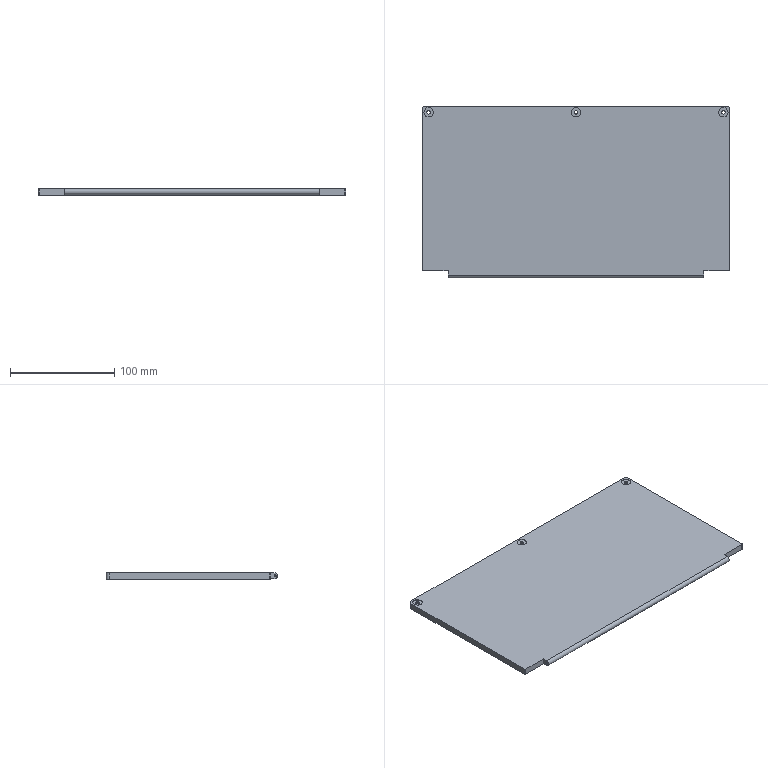NC program | Mastercam | posted with a generic post
Lines 3928 to 5159 of 5159:
N9570 T1 M6
N9580 G0 G90 G17 G54 X132.7 Y166.99 A0. S10000 M3
N9590 G43 H1 Z50. M8
N9600 Z.529
N9610 G1 Z-4.093 F600.
N9620 X122.7 F3000.
N9630 Z-4.471 F600.
N9640 X-122.7 F3000.
N9650 Z-4.093
N9660 X-132.7
N9670 Z-4.336
N9680 Y166.998
N9690 X-122.7
N9700 X122.7
N9710 X132.7
N9720 Z-4.2
N9730 Y167.
N9740 X122.7
N9750 X-122.7
N9760 X-132.7
N9770 Z-4.064
N9780 Y166.998
N9790 X-122.7
N9800 X122.7
N9810 X132.7
N9820 Z-3.929
N9830 Y166.99
N9840 X122.7
N9850 X-122.7
N9860 X-132.7
N9870 Z-3.794
N9880 Y166.978
N9890 X-122.7
N9900 X122.7
N9910 X132.7
N9920 Z-3.66
N9930 Y166.961
N9940 X122.7
N9950 X-122.7
N9960 X-132.7
N9970 Z-3.527
N9980 Y166.94
N9990 X-122.7
N100 X122.7
N110 X132.7
N120 Z-3.396
N130 Y166.914
N140 X122.7
N150 X-122.7
N160 X-132.7
N170 Z-3.265
N180 Y166.883
N190 X-122.7
N200 X122.7
N210 X132.7
N220 Z-3.137
N230 Y166.848
N240 X122.7
N250 X-122.7
N260 X-132.7
N270 Z-3.01
N280 Y166.809
N290 X-122.7
N300 X122.7
N310 X132.7
N320 Z-2.886
N330 Y166.765
N340 X122.7
N350 X-122.7
N360 X-132.7
N370 Z-2.764
N380 Y166.718
N390 X-122.7
N400 X122.7
N410 X132.7
N420 Z-2.644
N430 Y166.667
N440 X122.7
N450 X-122.7
N460 X-132.7
N470 Z-2.527
N480 Y166.612
N490 X-122.7
N500 X122.7
N510 X132.7
N520 Z-2.413
N530 Y166.554
N540 X122.7
N550 X-122.7
N560 X-132.7
N570 Z-2.302
N580 Y166.492
N590 X-122.7
N600 X122.7
N610 X132.7
N620 Z-2.194
N630 Y166.427
N640 X122.7
N650 X-122.7
N660 X-132.7
N670 Z-2.089
N680 Y166.36
N690 X-122.7
N700 X122.7
N710 X132.7
N720 Z-1.987
N730 Y166.289
N740 X122.7
N750 X-122.7
N760 X-132.7
N770 Z-1.889
N780 Y166.216
N790 X-122.7
N800 X122.7
N810 X132.7
N820 Z-1.794
N830 Y166.141
N840 X122.7
N850 X-122.7
N860 X-132.7
N870 Z-1.703
N880 Y166.064
N890 X-122.7
N900 X122.7
N910 X132.7
N920 Z-1.615
N930 Y165.985
N940 X122.7
N950 X-122.7
N960 X-132.7
N970 Z-1.53
N980 Y165.904
N990 X-122.7
N1000 X122.7
N1010 X132.7
N1020 Z-1.45
N1030 Y165.822
N1040 X122.7
N1050 X-122.7
N1060 X-132.7
N1070 Z-1.372
N1080 Y165.739
N1090 X-122.7
N1100 X122.7
N1110 X132.7
N1120 Z-1.299
N1130 Y165.654
N1140 X122.7
N1150 X-122.7
N1160 X-132.7
N1170 Z-1.228
N1180 Y165.568
N1190 X-122.7
N1200 X122.7
N1210 X132.7
N1220 Z-1.161
N1230 Y165.482
N1240 X122.7
N1250 X-122.7
N1260 X-132.7
N1270 Z-1.081
N1280 Y165.371
N1290 X-122.7
N1300 X122.7
N1310 X132.7
N1320 Z-1.006
N1330 Y165.259
N1340 X122.7
N1350 X-122.7
N1360 X-132.7
N1370 Z-.937
N1380 Y165.147
N1390 X-122.7
N1400 X122.7
N1410 X132.7
N1420 Z-.872
N1430 Y165.035
N1440 X122.7
N1450 X-122.7
N1460 X-132.7
N1470 Z-.813
N1480 Y164.923
N1490 X-122.7
N1500 X122.7
N1510 X132.7
N1520 Z-.758
N1530 Y164.811
N1540 X122.7
N1550 X-122.7
N1560 X-132.7
N1570 Z-.709
N1580 Y164.7
N1590 X-122.7
N1600 X122.7
N1610 X132.7
N1620 Z-.663
N1630 Y164.59
N1640 X122.7
N1650 X-122.7
N1660 X-132.7
N1670 Z-.622
N1680 Y164.48
N1690 X-122.7
N1700 X122.7
N1710 X132.7
N1720 Z-.585
N1730 Y164.372
N1740 X122.7
N1750 X-122.7
N1760 X-132.7
N1770 Z-.552
N1780 Y164.265
N1790 X-122.7
N1800 X122.7
N1810 X132.7
N1820 Z-.523
N1830 Y164.16
N1840 X122.7
N1850 X-122.7
N1860 X-132.7
N1870 Z-.498
N1880 Y164.056
N1890 X-122.7
N1900 X122.7
N1910 X132.7
N1920 Z-.475
N1930 Y163.953
N1940 X122.7
N1950 X-122.7
N1960 X-132.7
N1970 Z-.456
N1980 Y163.853
N1990 X-122.7
N2000 X122.7
N2010 X132.7
N2020 Z-.441
N2030 Y163.754
N2040 X122.7
N2050 X-122.7
N2060 X-132.7
N2070 Z-.428
N2080 Y163.657
N2090 X-122.7
N2100 X122.7
N2110 X132.7
N2120 Z-.417
N2130 Y163.561
N2140 X122.7
N2150 X-122.7
N2160 X-132.7
N2170 Z-.409
N2180 Y163.468
N2190 X-122.7
N2200 X122.7
N2210 X132.7
N2220 Z-.404
N2230 Y163.377
N2240 X122.7
N2250 X-122.7
N2260 X-132.7
N2270 Z-.401
N2280 Y163.287
N2290 X-122.7
N2300 X122.7
N2310 X132.7
N2320 Z-.4
N2330 Y163.2
N2340 X122.7
N2350 X-122.7
N2360 X-132.7
N2370 G0 Z4.6
N2380 Z50.
N2390 M5
N2400 G91 G28 Z0. M9
N2410 A0.
N2420 M01
N2430 T6 M6
N2440 G0 G90 G17 G54 X-134.7 Y161.1 A0. S7000 M3
N2450 G43 H6 Z50. M8
N2460 Z1.
N2470 G1 Z-.3 F600.
N2480 X-122.7 F3000.
N2490 X122.7
N2500 X134.7
N2510 G0 Z50.
N2520 X-134.7 Y161.
N2530 Z1.
N2540 G1 Z-.4 F600.
N2550 X-122.7 F1000.
N2560 X122.7
N2570 X134.7
N2580 G0 Z50.
N2590 M5
N2600 G91 G28 Z0. M9
N2610 A0.
N2620 M01
N2630 T3 M6
N2640 G0 G90 G17 G54 X0. Y6. A0. S7000 M3
N2650 G43 H3 Z50. M8
N2660 Z1.
N2670 G1 Z0. F600.
N2680 X.455 Y6.455 F2000.
N2690 G3 X0. Y6.91 I-.455 J0.
N2700 X-.91 Y6. Z-.05 I0. J-.91
N2710 X0. Y5.09 Z-.1 I.91 J0.
N2720 X.91 Y6. Z-.15 I0. J.91
N2730 X0. Y6.91 Z-.2 I-.91 J0.
N2740 X-.91 Y6. Z-.25 I0. J-.91
N2750 X0. Y5.09 Z-.3 I.91 J0.
N2760 X.91 Y6. Z-.35 I0. J.91
N2770 X0. Y6.91 Z-.4 I-.91 J0.
N2780 X-.91 Y6. Z-.45 I0. J-.91
N2790 X0. Y5.09 Z-.5 I.91 J0.
N2800 X.91 Y6. Z-.55 I0. J.91
N2810 X0. Y6.91 Z-.6 I-.91 J0.
N2820 X-.91 Y6. Z-.65 I0. J-.91
N2830 X0. Y5.09 Z-.7 I.91 J0.
N2840 X.91 Y6. Z-.75 I0. J.91
N2850 X0. Y6.91 Z-.8 I-.91 J0.
N2860 X-.91 Y6. Z-.85 I0. J-.91
N2870 X0. Y5.09 Z-.9 I.91 J0.
N2880 X.91 Y6. Z-.95 I0. J.91
N2890 X0. Y6.91 Z-1. I-.91 J0.
N2900 X-.91 Y6. Z-1.05 I0. J-.91
N2910 X0. Y5.09 Z-1.1 I.91 J0.
N2920 X.91 Y6. Z-1.15 I0. J.91
N2930 X0. Y6.91 Z-1.2 I-.91 J0.
N2940 X-.91 Y6. Z-1.25 I0. J-.91
N2950 X0. Y5.09 Z-1.3 I.91 J0.
N2960 X.91 Y6. Z-1.35 I0. J.91
N2970 X0. Y6.91 Z-1.4 I-.91 J0.
N2980 X-.91 Y6. Z-1.45 I0. J-.91
N2990 X0. Y5.09 Z-1.5 I.91 J0.
N3000 X.91 Y6. Z-1.55 I0. J.91
N3010 X0. Y6.91 Z-1.6 I-.91 J0.
N3020 X-.91 Y6. Z-1.65 I0. J-.91
N3030 X0. Y5.09 Z-1.7 I.91 J0.
N3040 X.91 Y6. Z-1.75 I0. J.91
N3050 X0. Y6.91 Z-1.8 I-.91 J0.
N3060 X-.91 Y6. Z-1.85 I0. J-.91
N3070 X0. Y5.09 Z-1.9 I.91 J0.
N3080 X.91 Y6. Z-1.95 I0. J.91
N3090 X0. Y6.91 Z-2. I-.91 J0.
N3100 X-.91 Y6. Z-2.05 I0. J-.91
N3110 X0. Y5.09 Z-2.1 I.91 J0.
N3120 X.91 Y6. Z-2.15 I0. J.91
N3130 X0. Y6.91 Z-2.2 I-.91 J0.
N3140 X-.91 Y6. Z-2.25 I0. J-.91
N3150 X0. Y5.09 Z-2.3 I.91 J0.
N3160 X.91 Y6. Z-2.35 I0. J.91
N3170 X0. Y6.91 Z-2.4 I-.91 J0.
N3180 X-.91 Y6. Z-2.45 I0. J-.91
N3190 X0. Y5.09 Z-2.5 I.91 J0.
N3200 X.91 Y6. Z-2.55 I0. J.91
N3210 X0. Y6.91 Z-2.6 I-.91 J0.
N3220 X-.91 Y6. Z-2.65 I0. J-.91
N3230 X0. Y5.09 Z-2.7 I.91 J0.
N3240 X.91 Y6. Z-2.75 I0. J.91
N3250 X0. Y6.91 Z-2.8 I-.91 J0.
N3260 X-.91 Y6. Z-2.85 I0. J-.91
N3270 X0. Y5.09 Z-2.9 I.91 J0.
N3280 X.91 Y6. Z-2.95 I0. J.91
N3290 X0. Y6.91 Z-3. I-.91 J0.
N3300 X-.91 Y6. Z-3.05 I0. J-.91
N3310 X0. Y5.09 Z-3.1 I.91 J0.
N3320 X.91 Y6. Z-3.15 I0. J.91
N3330 X0. Y6.91 Z-3.2 I-.91 J0.
N3340 X-.91 Y6. Z-3.25 I0. J-.91
N3350 X0. Y5.09 Z-3.3 I.91 J0.
N3360 X.91 Y6. Z-3.35 I0. J.91
N3370 X0. Y6.91 Z-3.4 I-.91 J0.
N3380 X-.91 Y6. Z-3.45 I0. J-.91
N3390 X0. Y5.09 Z-3.5 I.91 J0.
N3400 X.91 Y6. Z-3.55 I0. J.91
N3410 X0. Y6.91 Z-3.6 I-.91 J0.
N3420 X-.91 Y6. Z-3.65 I0. J-.91
N3430 X0. Y5.09 Z-3.7 I.91 J0.
N3440 X.91 Y6. Z-3.75 I0. J.91
N3450 X0. Y6.91 Z-3.8 I-.91 J0.
N3460 X-.91 Y6. Z-3.85 I0. J-.91
N3470 X0. Y5.09 Z-3.9 I.91 J0.
N3480 X.91 Y6. Z-3.95 I0. J.91
N3490 X0. Y6.91 Z-4. I-.91 J0.
N3500 X-.91 Y6. I0. J-.91 F1000.
N3510 X0. Y5.09 I.91 J0.
N3520 X.91 Y6. I0. J.91
N3530 X0. Y6.91 I-.91 J0.
N3540 X-.475 Y6.776 I0. J-.91
N3550 X-.693 Y6.388 I.237 J-.388
N3560 X-.626 Y6.15 I.455 J0.
N3570 G1 X0. Y6.
N3580 G0 Z0.
N3590 G1 X.505 Y6.505 F500.
N3600 G3 X0. Y7.01 I-.505 J0.
N3610 X-1.01 Y6. I0. J-1.01
N3620 X0. Y4.99 I1.01 J0.
N3630 X1.01 Y6. I0. J1.01
N3640 X0. Y7.01 I-1.01 J0.
N3650 X-.48 Y6.889 I0. J-1.01
N3660 X-1.01 Y6. Z-.514 I.48 J-.889
N3670 X0. Y4.99 Z-1.264 I1.01 J0.
N3680 X1.01 Y6. Z-2.014 I0. J1.01
N3690 X0. Y7.01 Z-2.764 I-1.01 J0.
N3700 X-.48 Y6.889 Z-3. I0. J-1.01
N3710 X-1.01 Y6. Z-3.514 I.48 J-.889
N3720 X-.53 Y5.14 Z-4. I1.01 J0.
N3730 X0. Y4.99 I.53 J.86
N3740 X1.01 Y6. I0. J1.01
N3750 X0. Y7.01 I-1.01 J0.
N3760 X-1.01 Y6. I0. J-1.01
N3770 X-.53 Y5.14 I1.01 J0.
N3780 X-.058 Y4.992 I.53 J.86
N3790 X-.029 Y4.991 I.029 J.504
N3800 X.475 Y5.467 I0. J.505
N3810 G1 X0. Y6.
N3820 G0 Z50.
N3830 X141.5
N3840 Z1.
N3850 G1 Z0. F600.
N3860 X141.955 Y6.455 F2000.
N3870 G3 X141.5 Y6.91 I-.455 J0.
N3880 X140.59 Y6. Z-.05 I0. J-.91
N3890 X141.5 Y5.09 Z-.1 I.91 J0.
N3900 X142.41 Y6. Z-.15 I0. J.91
N3910 X141.5 Y6.91 Z-.2 I-.91 J0.
N3920 X140.59 Y6. Z-.25 I0. J-.91
N3930 X141.5 Y5.09 Z-.3 I.91 J0.
N3940 X142.41 Y6. Z-.35 I0. J.91
N3950 X141.5 Y6.91 Z-.4 I-.91 J0.
N3960 X140.59 Y6. Z-.45 I0. J-.91
N3970 X141.5 Y5.09 Z-.5 I.91 J0.
N3980 X142.41 Y6. Z-.55 I0. J.91
N3990 X141.5 Y6.91 Z-.6 I-.91 J0.
N4000 X140.59 Y6. Z-.65 I0. J-.91
N4010 X141.5 Y5.09 Z-.7 I.91 J0.
N4020 X142.41 Y6. Z-.75 I0. J.91
N4030 X141.5 Y6.91 Z-.8 I-.91 J0.
N4040 X140.59 Y6. Z-.85 I0. J-.91
N4050 X141.5 Y5.09 Z-.9 I.91 J0.
N4060 X142.41 Y6. Z-.95 I0. J.91
N4070 X141.5 Y6.91 Z-1. I-.91 J0.
N4080 X140.59 Y6. Z-1.05 I0. J-.91
N4090 X141.5 Y5.09 Z-1.1 I.91 J0.
N4100 X142.41 Y6. Z-1.15 I0. J.91
N4110 X141.5 Y6.91 Z-1.2 I-.91 J0.
N4120 X140.59 Y6. Z-1.25 I0. J-.91
N4130 X141.5 Y5.09 Z-1.3 I.91 J0.
N4140 X142.41 Y6. Z-1.35 I0. J.91
N4150 X141.5 Y6.91 Z-1.4 I-.91 J0.
N4160 X140.59 Y6. Z-1.45 I0. J-.91
N4170 X141.5 Y5.09 Z-1.5 I.91 J0.
N4180 X142.41 Y6. Z-1.55 I0. J.91
N4190 X141.5 Y6.91 Z-1.6 I-.91 J0.
N4200 X140.59 Y6. Z-1.65 I0. J-.91
N4210 X141.5 Y5.09 Z-1.7 I.91 J0.
N4220 X142.41 Y6. Z-1.75 I0. J.91
N4230 X141.5 Y6.91 Z-1.8 I-.91 J0.
N4240 X140.59 Y6. Z-1.85 I0. J-.91
N4250 X141.5 Y5.09 Z-1.9 I.91 J0.
N4260 X142.41 Y6. Z-1.95 I0. J.91
N4270 X141.5 Y6.91 Z-2. I-.91 J0.
N4280 X140.59 Y6. Z-2.05 I0. J-.91
N4290 X141.5 Y5.09 Z-2.1 I.91 J0.
N4300 X142.41 Y6. Z-2.15 I0. J.91
N4310 X141.5 Y6.91 Z-2.2 I-.91 J0.
N4320 X140.59 Y6. Z-2.25 I0. J-.91
N4330 X141.5 Y5.09 Z-2.3 I.91 J0.
N4340 X142.41 Y6. Z-2.35 I0. J.91
N4350 X141.5 Y6.91 Z-2.4 I-.91 J0.
N4360 X140.59 Y6. Z-2.45 I0. J-.91
N4370 X141.5 Y5.09 Z-2.5 I.91 J0.
N4380 X142.41 Y6. Z-2.55 I0. J.91
N4390 X141.5 Y6.91 Z-2.6 I-.91 J0.
N4400 X140.59 Y6. Z-2.65 I0. J-.91
N4410 X141.5 Y5.09 Z-2.7 I.91 J0.
N4420 X142.41 Y6. Z-2.75 I0. J.91
N4430 X141.5 Y6.91 Z-2.8 I-.91 J0.
N4440 X140.59 Y6. Z-2.85 I0. J-.91
N4450 X141.5 Y5.09 Z-2.9 I.91 J0.
N4460 X142.41 Y6. Z-2.95 I0. J.91
N4470 X141.5 Y6.91 Z-3. I-.91 J0.
N4480 X140.59 Y6. Z-3.05 I0. J-.91
N4490 X141.5 Y5.09 Z-3.1 I.91 J0.
N4500 X142.41 Y6. Z-3.15 I0. J.91
N4510 X141.5 Y6.91 Z-3.2 I-.91 J0.
N4520 X140.59 Y6. Z-3.25 I0. J-.91
N4530 X141.5 Y5.09 Z-3.3 I.91 J0.
N4540 X142.41 Y6. Z-3.35 I0. J.91
N4550 X141.5 Y6.91 Z-3.4 I-.91 J0.
N4560 X140.59 Y6. Z-3.45 I0. J-.91
N4570 X141.5 Y5.09 Z-3.5 I.91 J0.
N4580 X142.41 Y6. Z-3.55 I0. J.91
N4590 X141.5 Y6.91 Z-3.6 I-.91 J0.
N4600 X140.59 Y6. Z-3.65 I0. J-.91
N4610 X141.5 Y5.09 Z-3.7 I.91 J0.
N4620 X142.41 Y6. Z-3.75 I0. J.91
N4630 X141.5 Y6.91 Z-3.8 I-.91 J0.
N4640 X140.59 Y6. Z-3.85 I0. J-.91
N4650 X141.5 Y5.09 Z-3.9 I.91 J0.
N4660 X142.41 Y6. Z-3.95 I0. J.91
N4670 X141.5 Y6.91 Z-4. I-.91 J0.
N4680 X140.59 Y6. I0. J-.91 F1000.
N4690 X141.5 Y5.09 I.91 J0.
N4700 X142.41 Y6. I0. J.91
N4710 X141.5 Y6.91 I-.91 J0.
N4720 X141.025 Y6.776 I0. J-.91
N4730 X140.807 Y6.388 I.237 J-.388
N4740 X140.874 Y6.15 I.455 J0.
N4750 G1 X141.5 Y6.
N4760 G0 Z0.
N4770 G1 X142.005 Y6.505 F500.
N4780 G3 X141.5 Y7.01 I-.505 J0.
N4790 X140.49 Y6. I0. J-1.01
N4800 X141.5 Y4.99 I1.01 J0.
N4810 X142.51 Y6. I0. J1.01
N4820 X141.5 Y7.01 I-1.01 J0.
N4830 X141.02 Y6.889 I0. J-1.01
N4840 X140.49 Y6. Z-.514 I.48 J-.889
N4850 X141.5 Y4.99 Z-1.264 I1.01 J0.
N4860 X142.51 Y6. Z-2.014 I0. J1.01
N4870 X141.5 Y7.01 Z-2.764 I-1.01 J0.
N4880 X141.02 Y6.889 Z-3. I0. J-1.01
N4890 X140.49 Y6. Z-3.514 I.48 J-.889
N4900 X140.97 Y5.14 Z-4. I1.01 J0.
N4910 X141.5 Y4.99 I.53 J.86
N4920 X142.51 Y6. I0. J1.01
N4930 X141.5 Y7.01 I-1.01 J0.
N4940 X140.49 Y6. I0. J-1.01
N4950 X140.97 Y5.14 I1.01 J0.
N4960 X141.442 Y4.992 I.53 J.86
N4970 X141.471 Y4.991 I.029 J.504
N4980 X141.975 Y5.467 I0. J.505
N4990 G1 X141.5 Y6.
N5000 G0 Z50.
N5010 X-141.5
N5020 Z1.
N5030 G1 Z0. F600.
N5040 X-141.045 Y6.455 F2000.
N5050 G3 X-141.5 Y6.91 I-.455 J0.
N5060 X-142.41 Y6. Z-.05 I0. J-.91
N5070 X-141.5 Y5.09 Z-.1 I.91 J0.
N5080 X-140.59 Y6. Z-.15 I0. J.91
N5090 X-141.5 Y6.91 Z-.2 I-.91 J0.
N5100 X-142.41 Y6. Z-.25 I0. J-.91
N5110 X-141.5 Y5.09 Z-.3 I.91 J0.
N5120 X-140.59 Y6. Z-.35 I0. J.91
N5130 X-141.5 Y6.91 Z-.4 I-.91 J0.
N5140 X-142.41 Y6. Z-.45 I0. J-.91
N5150 X-141.5 Y5.09 Z-.5 I.91 J0.
N5160 X-140.59 Y6. Z-.55 I0. J.91
N5170 X-141.5 Y6.91 Z-.6 I-.91 J0.
N5180 X-142.41 Y6. Z-.65 I0. J-.91
N5190 X-141.5 Y5.09 Z-.7 I.91 J0.
N5200 X-140.59 Y6. Z-.75 I0. J.91
N5210 X-141.5 Y6.91 Z-.8 I-.91 J0.
N5220 X-142.41 Y6. Z-.85 I0. J-.91
N5230 X-141.5 Y5.09 Z-.9 I.91 J0.
N5240 X-140.59 Y6. Z-.95 I0. J.91
N5250 X-141.5 Y6.91 Z-1. I-.91 J0.
N5260 X-142.41 Y6. Z-1.05 I0. J-.91
N5270 X-141.5 Y5.09 Z-1.1 I.91 J0.
N5280 X-140.59 Y6. Z-1.15 I0. J.91
N5290 X-141.5 Y6.91 Z-1.2 I-.91 J0.
N5300 X-142.41 Y6. Z-1.25 I0. J-.91
N5310 X-141.5 Y5.09 Z-1.3 I.91 J0.
N5320 X-140.59 Y6. Z-1.35 I0. J.91
N5330 X-141.5 Y6.91 Z-1.4 I-.91 J0.
N5340 X-142.41 Y6. Z-1.45 I0. J-.91
N5350 X-141.5 Y5.09 Z-1.5 I.91 J0.
N5360 X-140.59 Y6. Z-1.55 I0. J.91
N5370 X-141.5 Y6.91 Z-1.6 I-.91 J0.
N5380 X-142.41 Y6. Z-1.65 I0. J-.91
N5390 X-141.5 Y5.09 Z-1.7 I.91 J0.
N5400 X-140.59 Y6. Z-1.75 I0. J.91
N5410 X-141.5 Y6.91 Z-1.8 I-.91 J0.
N5420 X-142.41 Y6. Z-1.85 I0. J-.91
N5430 X-141.5 Y5.09 Z-1.9 I.91 J0.
N5440 X-140.59 Y6. Z-1.95 I0. J.91
N5450 X-141.5 Y6.91 Z-2. I-.91 J0.
N5460 X-142.41 Y6. Z-2.05 I0. J-.91
N5470 X-141.5 Y5.09 Z-2.1 I.91 J0.
N5480 X-140.59 Y6. Z-2.15 I0. J.91
N5490 X-141.5 Y6.91 Z-2.2 I-.91 J0.
N5500 X-142.41 Y6. Z-2.25 I0. J-.91
N5510 X-141.5 Y5.09 Z-2.3 I.91 J0.
N5520 X-140.59 Y6. Z-2.35 I0. J.91
N5530 X-141.5 Y6.91 Z-2.4 I-.91 J0.
N5540 X-142.41 Y6. Z-2.45 I0. J-.91
N5550 X-141.5 Y5.09 Z-2.5 I.91 J0.
N5560 X-140.59 Y6. Z-2.55 I0. J.91
N5570 X-141.5 Y6.91 Z-2.6 I-.91 J0.
N5580 X-142.41 Y6. Z-2.65 I0. J-.91
N5590 X-141.5 Y5.09 Z-2.7 I.91 J0.
N5600 X-140.59 Y6. Z-2.75 I0. J.91
N5610 X-141.5 Y6.91 Z-2.8 I-.91 J0.
N5620 X-142.41 Y6. Z-2.85 I0. J-.91
N5630 X-141.5 Y5.09 Z-2.9 I.91 J0.
N5640 X-140.59 Y6. Z-2.95 I0. J.91
N5650 X-141.5 Y6.91 Z-3. I-.91 J0.
N5660 X-142.41 Y6. Z-3.05 I0. J-.91
N5670 X-141.5 Y5.09 Z-3.1 I.91 J0.
N5680 X-140.59 Y6. Z-3.15 I0. J.91
N5690 X-141.5 Y6.91 Z-3.2 I-.91 J0.
N5700 X-142.41 Y6. Z-3.25 I0. J-.91
N5710 X-141.5 Y5.09 Z-3.3 I.91 J0.
N5720 X-140.59 Y6. Z-3.35 I0. J.91
N5730 X-141.5 Y6.91 Z-3.4 I-.91 J0.
N5740 X-142.41 Y6. Z-3.45 I0. J-.91
N5750 X-141.5 Y5.09 Z-3.5 I.91 J0.
N5760 X-140.59 Y6. Z-3.55 I0. J.91
N5770 X-141.5 Y6.91 Z-3.6 I-.91 J0.
N5780 X-142.41 Y6. Z-3.65 I0. J-.91
N5790 X-141.5 Y5.09 Z-3.7 I.91 J0.
N5800 X-140.59 Y6. Z-3.75 I0. J.91
N5810 X-141.5 Y6.91 Z-3.8 I-.91 J0.
N5820 X-142.41 Y6. Z-3.85 I0. J-.91
N5830 X-141.5 Y5.09 Z-3.9 I.91 J0.
N5840 X-140.59 Y6. Z-3.95 I0. J.91
N5850 X-141.5 Y6.91 Z-4. I-.91 J0.
N5860 X-142.41 Y6. I0. J-.91 F1000.
N5870 X-141.5 Y5.09 I.91 J0.
N5880 X-140.59 Y6. I0. J.91
N5890 X-141.5 Y6.91 I-.91 J0.
N5900 X-141.975 Y6.776 I0. J-.91
N5910 X-142.193 Y6.388 I.237 J-.388
N5920 X-142.126 Y6.15 I.455 J0.
N5930 G1 X-141.5 Y6.
N5940 G0 Z0.
N5950 G1 X-140.995 Y6.505 F500.
N5960 G3 X-141.5 Y7.01 I-.505 J0.
N5970 X-142.51 Y6. I0. J-1.01
N5980 X-141.5 Y4.99 I1.01 J0.
N5990 X-140.49 Y6. I0. J1.01
N6000 X-141.5 Y7.01 I-1.01 J0.
N6010 X-141.98 Y6.889 I0. J-1.01
N6020 X-142.51 Y6. Z-.514 I.48 J-.889
N6030 X-141.5 Y4.99 Z-1.264 I1.01 J0.
N6040 X-140.49 Y6. Z-2.014 I0. J1.01
N6050 X-141.5 Y7.01 Z-2.764 I-1.01 J0.
N6060 X-141.98 Y6.889 Z-3. I0. J-1.01
N6070 X-142.51 Y6. Z-3.514 I.48 J-.889
N6080 X-142.03 Y5.14 Z-4. I1.01 J0.
N6090 X-141.5 Y4.99 I.53 J.86
N6100 X-140.49 Y6. I0. J1.01
N6110 X-141.5 Y7.01 I-1.01 J0.
N6120 X-142.51 Y6. I0. J-1.01
N6130 X-142.03 Y5.14 I1.01 J0.
N6140 X-141.558 Y4.992 I.53 J.86
N6150 X-141.529 Y4.991 I.029 J.504
N6160 X-141.025 Y5.467 I0. J.505
N6170 G1 X-141.5 Y6.
N6180 G0 Z50.
N6190 M5
N6200 G91 G28 Z0. M9
N6210 A0.
N6220 M01
N6230 T5 M6
N6240 G0 G90 G17 G54 X146.1 Y159.45 A0. S7000 M3
N6250 G43 H5 Z50. M8
N6260 Z1.
N6270 G1 Z-.8 F600.
N6280 Y159.05 F1000.
N6290 G3 X146.5 Y158.65 I.4 J0.
N6300 G2 X148.15 Y157. I0. J-1.65
N6310 G1 Y3.
N6320 G2 X144.5 Y-.65 I-3.65 J0.
N6330 G1 X-144.5
N6340 G2 X-148.15 Y3. I0. J3.65
N6350 G1 Y157.
N6360 G2 X-146.5 Y158.65 I1.65 J0.
N6370 G3 X-146.1 Y159.05 I0. J.4
N6380 G1 Y159.45
N6390 G0 Z50.
N6400 X-140.45 Y5.6
N6410 Z1.
N6420 G1 Z-.8 F600.
N6430 X-140.05 F1000.
N6440 G3 X-139.65 Y6. I0. J.4
N6450 X-141.5 Y7.85 I-1.85 J0.
N6460 X-143.35 Y6. I0. J-1.85
N6470 X-141.5 Y4.15 I1.85 J0.
N6480 X-139.65 Y6. I0. J1.85
N6490 X-140.05 Y6.4 I-.4 J0.
N6500 G1 X-140.45
N6510 G0 Z50.
N6520 X1.05 Y5.6
N6530 Z1.
N6540 G1 Z-.8 F600.
N6550 X1.45 F1000.
N6560 G3 X1.85 Y6. I0. J.4
N6570 X0. Y7.85 I-1.85 J0.
N6580 X-1.85 Y6. I0. J-1.85
N6590 X0. Y4.15 I1.85 J0.
N6600 X1.85 Y6. I0. J1.85
N6610 X1.45 Y6.4 I-.4 J0.
N6620 G1 X1.05
N6630 G0 Z50.
N6640 X142.55 Y5.6
N6650 Z1.
N6660 G1 Z-.8 F600.
N6670 X142.95 F1000.
N6680 G3 X143.35 Y6. I0. J.4
N6690 X141.5 Y7.85 I-1.85 J0.
N6700 X139.65 Y6. I0. J-1.85
N6710 X141.5 Y4.15 I1.85 J0.
N6720 X143.35 Y6. I0. J1.85
N6730 X142.95 Y6.4 I-.4 J0.
N6740 G1 X142.55
N6750 G0 Z50.
N6760 X-141.313 Y152.379
N6770 Z1.
N6780 G1 Z-.8 F600.
N6790 X-141.596 Y152.662 F1000.
N6800 G3 X-141.879 Y152.779 I-.283 J-.283
N6810 X-142.162 Y152.662 I0. J-.4
N6820 X-142.85 Y151. I1.662 J-1.662
N6830 G1 Y15.243
N6840 G3 X-142.162 Y13.581 I2.35 J0.
N6850 G1 X-133.919 Y5.338
N6860 G3 X-132.257 Y4.65 I1.662 J1.662
N6870 G1 X-11.243
N6880 G3 X-9.581 Y5.338 I0. J2.35
N6890 G1 X-5.338 Y9.581
N6900 G2 X-2.757 Y10.65 I2.581 J-2.581
N6910 G1 X2.757
N6920 G2 X5.338 Y9.581 I0. J-3.65
N6930 G1 X9.581 Y5.338
N6940 G3 X11.243 Y4.65 I1.662 J1.662
N6950 G1 X132.257
N6960 G3 X133.919 Y5.338 I0. J2.35
N6970 G1 X142.162 Y13.581
N6980 G3 X142.85 Y15.243 I-1.662 J1.662
N6990 G1 Y151.
N7000 G3 X140.5 Y153.35 I-2.35 J0.
N7010 G1 X-140.5
N7020 G3 X-142.162 Y152.662 I0. J-2.35
N7030 X-142.279 Y152.379 I.283 J-.283
N7040 X-142.162 Y152.096 I.4 J0.
N7050 G1 X-141.879 Y151.813
N7060 G0 Z50.
N7070 X-146.9 Y159.1
N7080 Z1.
N7090 G1 Z-.3 F600.
N7100 Y158.7 F1000.
N7110 G3 X-146.5 Y158.3 I.4 J0.
N7120 G1 X146.5
N7130 G3 X146.9 Y158.7 I0. J.4
N7140 G1 Y159.1
N7150 G0 Z50.
N7160 M5
N7170 G91 G28 Z0. M9
N7180 A0.
N7190 M01
N7200 T8 M6
N7210 G0 G90 G17 G54 X4.1 Y8. A0. S7000 M3
N7220 G43 H8 Z50. M8
N7230 Z1.
N7240 G1 Z-.494 F600.
N7250 Y0. F3000.
N7260 Y-5.6
N7270 Y-13.6
N7280 Z-.988 F600.
N7290 Y-5.6 F3000.
N7300 Y0.
N7310 Y8.
N7320 Z-1.482 F600.
N7330 Y0. F3000.
N7340 Y-5.6
N7350 Y-13.6
N7360 Z-1.976 F600.
N7370 Y-5.6 F3000.
N7380 Y0.
N7390 Y8.
N7400 Z-2.47 F600.
N7410 Y0. F3000.
N7420 Y-5.6
N7430 Y-13.6
N7440 Z-2.964 F600.
N7450 Y-5.6 F3000.
N7460 Y0.
N7470 Y8.
N7480 Z-3.458 F600.
N7490 Y0. F3000.
N7500 Y-5.6
N7510 Y-13.6
N7520 Z-3.952 F600.
N7530 Y-5.6 F3000.
N7540 Y0.
N7550 Y8.
N7560 Z-4.446 F600.
N7570 Y0. F3000.
N7580 Y-5.6
N7590 Y-13.6
N7600 Z-4.94 F600.
N7610 Y-5.6 F3000.
N7620 Y0.
N7630 Y8.
N7640 Z-5.434 F600.
N7650 Y0. F3000.
N7660 Y-5.6
N7670 Y-13.6
N7680 Z-5.928 F600.
N7690 Y-5.6 F3000.
N7700 Y0.
N7710 Y8.
N7720 Z-6.422 F600.
N7730 Y0. F3000.
N7740 Y-5.6
N7750 Y-13.6
N7760 Z-6.916 F600.
N7770 Y-5.6 F3000.
N7780 Y0.
N7790 Y8.
N7800 Z-7.41 F600.
N7810 Y0. F3000.
N7820 Y-5.6
N7830 Y-13.6
N7840 Z-7.904 F600.
N7850 Y-5.6 F3000.
N7860 Y0.
N7870 Y8.
N7880 Z-8.398 F600.
N7890 Y0. F3000.
N7900 Y-5.6
N7910 Y-13.6
N7920 Z-8.892 F600.
N7930 Y-5.6 F3000.
N7940 Y0.
N7950 Y8.
N7960 Z-9.386 F600.
N7970 Y0. F3000.
N7980 Y-5.6
N7990 Y-13.6
N8000 Z-9.88 F600.
N8010 Y-5.6 F3000.
N8020 Y0.
N8030 Y8.
N8040 Z-10.374 F600.
N8050 Y0. F3000.
N8060 Y-5.6
N8070 Y-13.6
N8080 Z-10.868 F600.
N8090 Y-5.6 F3000.
N8100 Y0.
N8110 Y8.
N8120 Z-11.362 F600.
N8130 Y0. F3000.
N8140 Y-5.6
N8150 Y-13.6
N8160 Z-11.856 F600.
N8170 Y-5.6 F3000.
N8180 Y0.
N8190 Y8.
N8200 Z-12.35 F600.
N8210 Y0. F3000.
N8220 Y-5.6
N8230 Y-13.6
N8240 Z-12.844 F600.
N8250 Y-5.6 F3000.
N8260 Y0.
N8270 Y8.
N8280 Z-13.338 F600.
N8290 Y0. F3000.
N8300 Y-5.6
N8310 Y-13.6
N8320 Z-13.832 F600.
N8330 Y-5.6 F3000.
N8340 Y0.
N8350 Y8.
N8360 Z-14.326 F600.
N8370 Y0. F3000.
N8380 Y-5.6
N8390 Y-13.6
N8400 Z-14.82 F600.
N8410 Y-5.6 F3000.
N8420 Y0.
N8430 Y8.
N8440 Z-15.314 F600.
N8450 Y0. F3000.
N8460 Y-5.6
N8470 Y-13.6
N8480 Z-15.808 F600.
N8490 Y-5.6 F3000.
N8500 Y0.
N8510 Y8.
N8520 Z-16.302 F600.
N8530 Y0. F3000.
N8540 Y-5.6
N8550 Y-13.6
N8560 Z-16.796 F600.
N8570 Y-5.6 F3000.
N8580 Y0.
N8590 Y8.
N8600 Z-17.29 F600.
N8610 Y0. F3000.
N8620 Y-5.6
N8630 Y-13.6
N8640 Z-17.784 F600.
N8650 Y-5.6 F3000.
N8660 Y0.
N8670 Y8.
N8680 Z-18.278 F600.
N8690 Y0. F3000.
N8700 Y-5.6
N8710 Y-13.6
N8720 Z-18.772 F600.
N8730 Y-5.6 F3000.
N8740 Y0.
N8750 Y8.
N8760 Z-19.266 F600.
N8770 Y0. F3000.
N8780 Y-5.6
N8790 Y-13.6
N8800 Z-19.76 F600.
N8810 Y-5.6 F3000.
N8820 Y0.
N8830 Y8.
N8840 Z-20.254 F600.
N8850 Y0. F3000.
N8860 Y-5.6
N8870 Y-13.6
N8880 Z-20.748 F600.
N8890 Y-5.6 F3000.
N8900 Y0.
N8910 Y8.
N8920 Z-21.242 F600.
N8930 Y0. F3000.
N8940 Y-5.6
N8950 Y-13.6
N8960 Z-21.736 F600.
N8970 Y-5.6 F3000.
N8980 Y0.
N8990 Y8.
N9000 Z-22.23 F600.
N9010 Y0. F3000.
N9020 Y-5.6
N9030 Y-13.6
N9040 Z-22.724 F600.
N9050 Y-5.6 F3000.
N9060 Y0.
N9070 Y8.
N9080 Z-23.218 F600.
N9090 Y0. F3000.
N9100 Y-5.6
N9110 Y-13.6
N9120 Z-23.712 F600.
N9130 Y-5.6 F3000.
N9140 Y0.
N9150 Y8.
N9160 Z-24.206 F600.
N9170 Y0. F3000.
N9180 Y-5.6
N9190 Y-13.6
N9200 Z-24.7 F600.
N9210 Y-5.6 F3000.
N9220 Y0.
N9230 Y8.
N9240 G0 Z50.
N9250 X4.
N9260 Z1.
N9270 G1 Z-8.267 F600.
N9280 Y0. F1000.
N9290 Y-5.6
N9300 Y-13.6
N9310 G0 Z50.
N9320 Y8.
N9330 Z-7.267
N9340 G1 Z-16.533 F600.
N9350 Y0. F1000.
N9360 Y-5.6
N9370 Y-13.6
N9380 G0 Z50.
N9390 Y8.
N9400 Z-15.533
N9410 G1 Z-24.8 F600.
N9420 Y0. F1000.
N9430 Y-5.6
N9440 Y-13.6
N9450 G0 Z50.
N9460 M5
N9470 G91 G28 Z0. M9
N9480 A0.
N9490 M01
N9500 T5 M6
N9510 G0 G90 G17 G54 X4.2 Y-2.8 A0. S3000 M3
N9520 G43 H5 Z25.2 M8
N9530 G98 G81 Z-25.5 R-23.8 F300.
N9540 G80
N9550 M5
N9560 G91 G0 G28 Z0. M9
N9570 A0.
N9580 M01
N9590 T8 M6
N9600 G0 G90 G17 G54 X-4.1 Y-14. A0. S7000 M3
N9610 G43 H8 Z50. M8
N9620 Z1.
N9630 G1 Z-.494 F600.
N9640 Y-6. F3000.
N9650 Y0.
N9660 Y8.
N9670 Z-.988 F600.
N9680 Y0. F3000.
N9690 Y-6.
N9700 Y-14.
N9710 Z-1.482 F600.
N9720 Y-6. F3000.
N9730 Y0.
N9740 Y8.
N9750 Z-1.976 F600.
N9760 Y0. F3000.
N9770 Y-6.
N9780 Y-14.
N9790 Z-2.47 F600.
N9800 Y-6. F3000.
N9810 Y0.
N9820 Y8.
N9830 Z-2.964 F600.
N9840 Y0. F3000.
N9850 Y-6.
N9860 Y-14.
N9870 Z-3.458 F600.
N9880 Y-6. F3000.
N9890 Y0.
N9900 Y8.
N9910 Z-3.952 F600.
N9920 Y0. F3000.
N9930 Y-6.
N9940 Y-14.
N9950 Z-4.446 F600.
N9960 Y-6. F3000.
N9970 Y0.
N9980 Y8.
N9990 Z-4.94 F600.
N100 Y0. F3000.
N110 Y-6.
N120 Y-14.
N130 Z-5.434 F600.
N140 Y-6. F3000.
N150 Y0.
N160 Y8.
N170 Z-5.928 F600.
N180 Y0. F3000.
N190 Y-6.
N200 Y-14.
N210 Z-6.422 F600.
N220 Y-6. F3000.
N230 Y0.
N240 Y8.
N250 Z-6.916 F600.
N260 Y0. F3000.
N270 Y-6.
N280 Y-14.
N290 Z-7.41 F600.
N300 Y-6. F3000.
N310 Y0.
N320 Y8.
N330 Z-7.904 F600.
N340 Y0. F3000.
N350 Y-6.
N360 Y-14.
N370 Z-8.398 F600.
N380 Y-6. F3000.
N390 Y0.
N400 Y8.
N410 Z-8.892 F600.
N420 Y0. F3000.
N430 Y-6.
N440 Y-14.
N450 Z-9.386 F600.
N460 Y-6. F3000.
N470 Y0.
N480 Y8.
N490 Z-9.88 F600.
N500 Y0. F3000.
N510 Y-6.
N520 Y-14.
N530 Z-10.374 F600.
N540 Y-6. F3000.
N550 Y0.
N560 Y8.
N570 Z-10.868 F600.
N580 Y0. F3000.
N590 Y-6.
N600 Y-14.
N610 Z-11.362 F600.
N620 Y-6. F3000.
N630 Y0.
N640 Y8.
N650 Z-11.856 F600.
N660 Y0. F3000.
N670 Y-6.
N680 Y-14.
N690 Z-12.35 F600.
N700 Y-6. F3000.
N710 Y0.
N720 Y8.
N730 Z-12.844 F600.
N740 Y0. F3000.
N750 Y-6.
N760 Y-14.
N770 Z-13.338 F600.
N780 Y-6. F3000.
N790 Y0.
N800 Y8.
N810 Z-13.832 F600.
N820 Y0. F3000.
N830 Y-6.
N840 Y-14.
N850 Z-14.326 F600.
N860 Y-6. F3000.
N870 Y0.
N880 Y8.
N890 Z-14.82 F600.
N900 Y0. F3000.
N910 Y-6.
N920 Y-14.
N930 Z-15.314 F600.
N940 Y-6. F3000.
N950 Y0.
N960 Y8.
N970 Z-15.808 F600.
N980 Y0. F3000.
N990 Y-6.
N1000 Y-14.
N1010 Z-16.302 F600.
N1020 Y-6. F3000.
N1030 Y0.
N1040 Y8.
N1050 Z-16.796 F600.
N1060 Y0. F3000.
N1070 Y-6.
N1080 Y-14.
N1090 Z-17.29 F600.
N1100 Y-6. F3000.
N1110 Y0.
N1120 Y8.
N1130 Z-17.784 F600.
N1140 Y0. F3000.
N1150 Y-6.
N1160 Y-14.
N1170 Z-18.278 F600.
N1180 Y-6. F3000.
N1190 Y0.
N1200 Y8.
N1210 Z-18.772 F600.
N1220 Y0. F3000.
N1230 Y-6.
N1240 Y-14.
N1250 Z-19.266 F600.
N1260 Y-6. F3000.
N1270 Y0.
N1280 Y8.
N1290 Z-19.76 F600.
N1300 Y0. F3000.
N1310 Y-6.
N1320 Y-14.
N1330 Z-20.254 F600.
N1340 Y-6. F3000.
N1350 Y0.
N1360 Y8.
N1370 Z-20.748 F600.
N1380 Y0. F3000.
N1390 Y-6.
N1400 Y-14.
N1410 Z-21.242 F600.
N1420 Y-6. F3000.
N1430 Y0.
N1440 Y8.
N1450 Z-21.736 F600.
N1460 Y0. F3000.
N1470 Y-6.
N1480 Y-14.
N1490 Z-22.23 F600.
N1500 Y-6. F3000.
N1510 Y0.
N1520 Y8.
N1530 Z-22.724 F600.
N1540 Y0. F3000.
N1550 Y-6.
N1560 Y-14.
N1570 Z-23.218 F600.
N1580 Y-6. F3000.
N1590 Y0.
N1600 Y8.
N1610 Z-23.712 F600.
N1620 Y0. F3000.
N1630 Y-6.
N1640 Y-14.
N1650 Z-24.206 F600.
N1660 Y-6. F3000.
N1670 Y0.
N1680 Y8.
N1690 Z-24.7 F600.
N1700 Y0. F3000.
N1710 Y-6.
N1720 Y-14.
N1730 G0 Z50.
N1740 X-4.
N1750 Z1.
N1760 G1 Z-8.267 F600.
N1770 Y-6. F1000.
N1780 Y0.
N1790 Y8.
N1800 G0 Z50.
N1810 Y-14.
N1820 Z-7.267
N1830 G1 Z-16.533 F600.
N1840 Y-6. F1000.
N1850 Y0.
N1860 Y8.
N1870 G0 Z50.
N1880 Y-14.
N1890 Z-15.533
N1900 G1 Z-24.8 F600.
N1910 Y-6. F1000.
N1920 Y0.
N1930 Y8.
N1940 G0 Z50.
N1950 M5
N1960 G91 G28 Z0. M9
N1970 A0.
N1980 M01
N1990 T5 M6
N2000 G0 G90 G17 G54 X-4.2 Y-2.8 A0. S3000 M3
N2010 G43 H5 Z25.2 M8
N2020 G98 G81 Z-25.5 R-23.8 F300.
N2030 G80
N2040 M5
N2050 G91 G0 G28 Z0. M9
N2060 G28 X0. Y0. A0.
N2070 M30
%